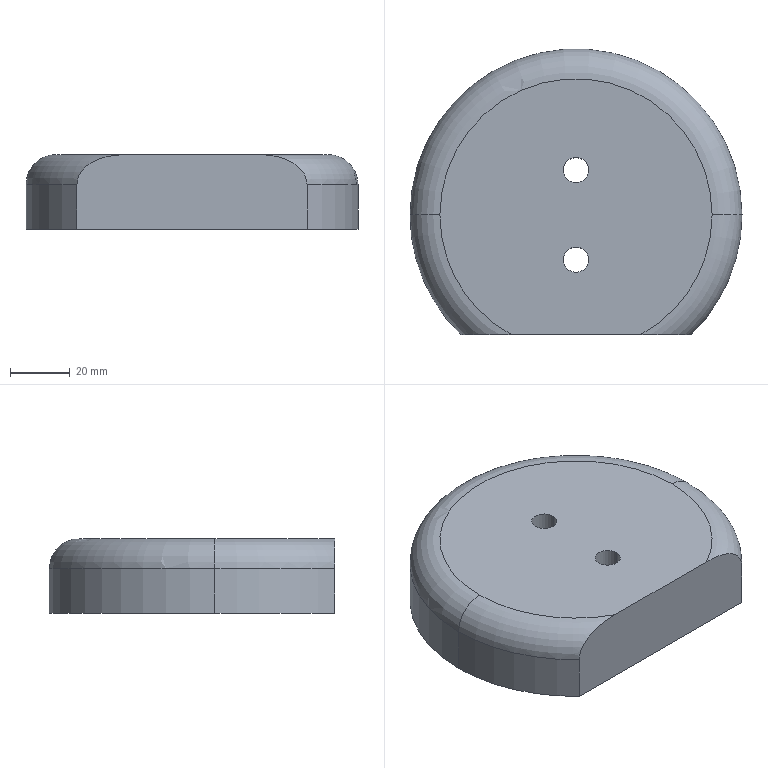Part | SolidWorks | features BaseBody 1 | 1 solid | 13 faces | box 111 x 95.5 x 25 mm | volume 213112 mm3 | cylinder 7 | plane 3 | torus 3 | commonest cylinder face diameters 8.4 x4 111 x3
STEP:
#1=CARTESIAN_POINT('',(-38.474,-40.,0.));
#2=VERTEX_POINT('',#1);
#3=CARTESIAN_POINT('',(38.474,-40.,0.));
#4=VERTEX_POINT('',#3);
#5=CARTESIAN_POINT('',(38.474,-40.,0.));
#6=DIRECTION('',(1.,0.,0.));
#7=VECTOR('',#6,1000.);
#8=LINE('',#5,#7);
#9=EDGE_CURVE('',#2,#4,#8,.T.);
#10=ORIENTED_EDGE('',*,*,#9,.T.);
#11=CARTESIAN_POINT('',(38.474,-40.,15.));
#12=VERTEX_POINT('',#11);
#13=CARTESIAN_POINT('',(38.474,-40.,-0.001));
#14=DIRECTION('',(0.,0.,1.));
#15=VECTOR('',#14,1000.);
#16=LINE('',#13,#15);
#17=EDGE_CURVE('',#4,#12,#16,.T.);
#18=ORIENTED_EDGE('',*,*,#17,.T.);
#19=CARTESIAN_POINT('',(21.685,-40.,25.));
#20=VERTEX_POINT('',#19);
#21=CARTESIAN_POINT('',(21.685,-40.,25.));
#22=CARTESIAN_POINT('',(22.606,-40.,25.));
#23=CARTESIAN_POINT('',(23.513,-40.,24.971));
#24=CARTESIAN_POINT('',(24.849,-40.,24.876));
#25=CARTESIAN_POINT('',(25.29,-40.,24.835));
#26=CARTESIAN_POINT('',(25.945,-40.,24.761));
#27=CARTESIAN_POINT('',(26.271,-40.,24.72));
#28=CARTESIAN_POINT('',(26.647,-40.,24.666));
#29=CARTESIAN_POINT('',(26.835,-40.,24.638));
#30=CARTESIAN_POINT('',(26.929,-40.,24.623));
#31=CARTESIAN_POINT('',(26.969,-40.,24.617));
#32=CARTESIAN_POINT('',(26.995,-40.,24.612));
#33=CARTESIAN_POINT('',(27.007,-40.,24.61));
#34=CARTESIAN_POINT('',(27.961,-40.,24.456));
#35=CARTESIAN_POINT('',(28.867,-40.,24.258));
#36=CARTESIAN_POINT('',(30.166,-40.,23.885));
#37=CARTESIAN_POINT('',(30.589,-40.,23.748));
#38=CARTESIAN_POINT('',(31.206,-40.,23.523));
#39=CARTESIAN_POINT('',(31.511,-40.,23.406));
#40=CARTESIAN_POINT('',(31.858,-40.,23.261));
#41=CARTESIAN_POINT('',(32.03,-40.,23.186));
#42=CARTESIAN_POINT('',(32.115,-40.,23.148));
#43=CARTESIAN_POINT('',(32.151,-40.,23.132));
#44=CARTESIAN_POINT('',(32.176,-40.,23.121));
#45=CARTESIAN_POINT('',(32.186,-40.,23.117));
#46=CARTESIAN_POINT('',(33.089,-40.,22.708));
#47=CARTESIAN_POINT('',(33.906,-40.,22.241));
#48=CARTESIAN_POINT('',(35.002,-40.,21.449));
#49=CARTESIAN_POINT('',(35.345,-40.,21.17));
#50=CARTESIAN_POINT('',(35.825,-40.,20.731));
#51=CARTESIAN_POINT('',(35.978,-40.,20.581));
#52=CARTESIAN_POINT('',(36.2,-40.,20.351));
#53=CARTESIAN_POINT('',(36.309,-40.,20.234));
#54=CARTESIAN_POINT('',(36.431,-40.,20.097));
#55=CARTESIAN_POINT('',(36.491,-40.,20.027));
#56=CARTESIAN_POINT('',(36.517,-40.,19.997));
#57=CARTESIAN_POINT('',(36.534,-40.,19.977));
#58=CARTESIAN_POINT('',(36.542,-40.,19.969));
#59=CARTESIAN_POINT('',(36.855,-40.,19.598));
#60=CARTESIAN_POINT('',(37.126,-40.,19.224));
#61=CARTESIAN_POINT('',(37.478,-40.,18.645));
#62=CARTESIAN_POINT('',(37.587,-40.,18.449));
#63=CARTESIAN_POINT('',(37.736,-40.,18.151));
#64=CARTESIAN_POINT('',(37.808,-40.,18.001));
#65=CARTESIAN_POINT('',(37.885,-40.,17.824));
#66=CARTESIAN_POINT('',(37.917,-40.,17.748));
#67=CARTESIAN_POINT('',(37.938,-40.,17.697));
#68=CARTESIAN_POINT('',(37.947,-40.,17.673));
#69=CARTESIAN_POINT('',(38.3,-40.,16.789));
#70=CARTESIAN_POINT('',(38.474,-40.,15.896));
#71=CARTESIAN_POINT('',(38.474,-40.,15.));
#72=B_SPLINE_CURVE_WITH_KNOTS('',3,(#21,#22,#23,#24,#25,#26,#27,#28,#29,#30,#31,#32,#33,#34,#35,#36,#37,#38,#39,#40,#41,#42,#43,#44,#45,#46,#47,#48,#49,#50,#51,#52,#53,#54,#55,#56,#57,#58,#59,#60,#61,#62,#63,#64,#65,#66,#67,#68,#69,#70,#71),.UNSPECIFIED.,.F.,.F.,(4,2,2,1,1,1,1,2,2,2,2,1,1,1,1,2,2,2,2,2,1,1,1,2,2,2,2,1,1,2,2,4),(0.,0.125,0.1875,0.2188,0.2344,0.2422,0.2461,0.248,0.25,0.375,0.4375,0.4688,0.4844,0.4922,0.4961,0.498,0.5,0.625,0.6875,0.7188,0.7344,0.7422,0.7461,0.748,0.75,0.8125,0.8437,0.8594,0.8672,0.8711,0.875,1.),.UNSPECIFIED.);
#73=EDGE_CURVE('',#20,#12,#72,.T.);
#74=ORIENTED_EDGE('',*,*,#73,.F.);
#75=CARTESIAN_POINT('',(-21.685,-40.,25.));
#76=VERTEX_POINT('',#75);
#77=CARTESIAN_POINT('',(38.474,-40.,25.));
#78=DIRECTION('',(-1.,0.,0.));
#79=VECTOR('',#78,1000.);
#80=LINE('',#77,#79);
#81=EDGE_CURVE('',#20,#76,#80,.T.);
#82=ORIENTED_EDGE('',*,*,#81,.T.);
#83=CARTESIAN_POINT('',(-38.474,-40.,15.));
#84=VERTEX_POINT('',#83);
#85=CARTESIAN_POINT('',(-38.474,-40.,15.));
#86=CARTESIAN_POINT('',(-38.474,-40.,15.879));
#87=CARTESIAN_POINT('',(-38.308,-39.999,16.75));
#88=CARTESIAN_POINT('',(-37.82,-39.999,18.005));
#89=CARTESIAN_POINT('',(-37.618,-39.999,18.414));
#90=CARTESIAN_POINT('',(-37.258,-40.,19.01));
#91=CARTESIAN_POINT('',(-37.128,-40.,19.205));
#92=CARTESIAN_POINT('',(-36.92,-40.,19.494));
#93=CARTESIAN_POINT('',(-36.813,-40.,19.636));
#94=CARTESIAN_POINT('',(-36.681,-40.,19.801));
#95=CARTESIAN_POINT('',(-36.614,-40.,19.882));
#96=CARTESIAN_POINT('',(-36.585,-40.,19.917));
#97=CARTESIAN_POINT('',(-36.566,-40.,19.94));
#98=CARTESIAN_POINT('',(-36.554,-40.,19.953));
#99=CARTESIAN_POINT('',(-36.004,-40.,20.603));
#100=CARTESIAN_POINT('',(-35.36,-40.,21.191));
#101=CARTESIAN_POINT('',(-34.263,-40.,21.982));
#102=CARTESIAN_POINT('',(-33.876,-40.,22.231));
#103=CARTESIAN_POINT('',(-33.265,-40.,22.58));
#104=CARTESIAN_POINT('',(-33.057,-40.,22.693));
#105=CARTESIAN_POINT('',(-32.737,-40.,22.856));
#106=CARTESIAN_POINT('',(-32.575,-40.,22.936));
#107=CARTESIAN_POINT('',(-32.383,-40.,23.026));
#108=CARTESIAN_POINT('',(-32.287,-40.,23.071));
#109=CARTESIAN_POINT('',(-32.245,-40.,23.09));
#110=CARTESIAN_POINT('',(-32.217,-40.,23.102));
#111=CARTESIAN_POINT('',(-32.202,-40.,23.109));
#112=CARTESIAN_POINT('',(-31.415,-40.,23.465));
#113=CARTESIAN_POINT('',(-30.591,-40.,23.763));
#114=CARTESIAN_POINT('',(-29.294,-40.,24.135));
#115=CARTESIAN_POINT('',(-28.852,-40.,24.247));
#116=CARTESIAN_POINT('',(-28.175,-40.,24.396));
#117=CARTESIAN_POINT('',(-27.833,-40.,24.466));
#118=CARTESIAN_POINT('',(-27.428,-40.,24.54));
#119=CARTESIAN_POINT('',(-27.224,-40.,24.575));
#120=CARTESIAN_POINT('',(-27.122,-40.,24.592));
#121=CARTESIAN_POINT('',(-27.078,-40.,24.599));
#122=CARTESIAN_POINT('',(-27.049,-40.,24.604));
#123=CARTESIAN_POINT('',(-27.033,-40.,24.606));
#124=CARTESIAN_POINT('',(-25.314,-40.,24.884));
#125=CARTESIAN_POINT('',(-23.527,-40.,25.));
#126=CARTESIAN_POINT('',(-21.685,-40.,25.));
#127=B_SPLINE_CURVE_WITH_KNOTS('',3,(#85,#86,#87,#88,#89,#90,#91,#92,#93,#94,#95,#96,#97,#98,#99,#100,#101,#102,#103,#104,#105,#106,#107,#108,#109,#110,#111,#112,#113,#114,#115,#116,#117,#118,#119,#120,#121,#122,#123,#124,#125,#126),.UNSPECIFIED.,.F.,.F.,(4,2,2,2,1,1,1,2,2,2,2,2,1,1,1,2,2,2,2,1,1,1,1,2,2,4),(0.,0.125,0.1875,0.2187,0.2344,0.2422,0.2461,0.248,0.25,0.375,0.4375,0.4687,0.4844,0.4922,0.4961,0.498,0.5,0.625,0.6875,0.7187,0.7344,0.7422,0.7461,0.748,0.75,1.),.UNSPECIFIED.);
#128=EDGE_CURVE('',#84,#76,#127,.T.);
#129=ORIENTED_EDGE('',*,*,#128,.F.);
#130=CARTESIAN_POINT('',(-38.474,-40.,-0.001));
#131=DIRECTION('',(0.,0.,1.));
#132=VECTOR('',#131,1000.);
#133=LINE('',#130,#132);
#134=EDGE_CURVE('',#2,#84,#133,.T.);
#135=ORIENTED_EDGE('',*,*,#134,.F.);
#136=EDGE_LOOP('',(#10,#18,#74,#82,#129,#135));
#137=FACE_OUTER_BOUND('',#136,.T.);
#138=CARTESIAN_POINT('',(38.474,-40.,-0.001));
#139=DIRECTION('',(0.,1.,0.));
#140=DIRECTION('',(1.,0.,0.));
#141=AXIS2_PLACEMENT_3D('',#138,#139,#140);
#142=PLANE('',#141);
#143=ADVANCED_FACE('',(#137),#142,.F.);
#144=CARTESIAN_POINT('',(-55.5,0.,15.));
#145=VERTEX_POINT('',#144);
#146=CARTESIAN_POINT('',(-45.5,0.,25.));
#147=VERTEX_POINT('',#146);
#148=CARTESIAN_POINT('',(-45.5,0.,15.));
#149=DIRECTION('',(0.,1.,0.));
#150=DIRECTION('',(-1.,0.,0.));
#151=AXIS2_PLACEMENT_3D('',#148,#149,#150);
#152=CIRCLE('',#151,10.);
#153=EDGE_CURVE('',#145,#147,#152,.T.);
#154=ORIENTED_EDGE('',*,*,#153,.F.);
#155=CARTESIAN_POINT('',(0.,0.,15.));
#156=DIRECTION('',(0.,0.,-1.));
#157=DIRECTION('',(1.,0.,0.));
#158=AXIS2_PLACEMENT_3D('',#155,#156,#157);
#159=CIRCLE('',#158,55.5);
#160=EDGE_CURVE('',#84,#145,#159,.T.);
#161=ORIENTED_EDGE('',*,*,#160,.F.);
#162=ORIENTED_EDGE('',*,*,#128,.T.);
#163=CARTESIAN_POINT('',(0.,0.,25.));
#164=DIRECTION('',(0.,0.,1.));
#165=DIRECTION('',(1.,0.,0.));
#166=AXIS2_PLACEMENT_3D('',#163,#164,#165);
#167=CIRCLE('',#166,45.5);
#168=EDGE_CURVE('',#147,#76,#167,.T.);
#169=ORIENTED_EDGE('',*,*,#168,.F.);
#170=EDGE_LOOP('',(#154,#161,#162,#169));
#171=FACE_OUTER_BOUND('',#170,.T.);
#172=CARTESIAN_POINT('',(0.,0.,15.));
#173=DIRECTION('',(0.,0.,1.));
#174=DIRECTION('',(1.,0.,0.));
#175=AXIS2_PLACEMENT_3D('',#172,#173,#174);
#176=TOROIDAL_SURFACE('',#175,45.5,10.);
#177=ADVANCED_FACE('',(#171),#176,.T.);
#178=CARTESIAN_POINT('',(-4.2,-15.,0.));
#179=VERTEX_POINT('',#178);
#180=CARTESIAN_POINT('',(-4.2,-15.,25.));
#181=VERTEX_POINT('',#180);
#182=CARTESIAN_POINT('',(-4.2,-15.,25.));
#183=DIRECTION('',(0.,0.,1.));
#184=VECTOR('',#183,1000.);
#185=LINE('',#182,#184);
#186=EDGE_CURVE('',#179,#181,#185,.T.);
#187=ORIENTED_EDGE('',*,*,#186,.F.);
#188=CARTESIAN_POINT('',(4.2,-15.,0.));
#189=VERTEX_POINT('',#188);
#190=CARTESIAN_POINT('',(0.,-15.,0.));
#191=DIRECTION('',(0.,0.,1.));
#192=DIRECTION('',(1.,0.,0.));
#193=AXIS2_PLACEMENT_3D('',#190,#191,#192);
#194=CIRCLE('',#193,4.2);
#195=EDGE_CURVE('',#189,#179,#194,.T.);
#196=ORIENTED_EDGE('',*,*,#195,.F.);
#197=CARTESIAN_POINT('',(4.2,-15.,25.));
#198=VERTEX_POINT('',#197);
#199=CARTESIAN_POINT('',(4.2,-15.,25.));
#200=DIRECTION('',(0.,0.,1.));
#201=VECTOR('',#200,1000.);
#202=LINE('',#199,#201);
#203=EDGE_CURVE('',#189,#198,#202,.T.);
#204=ORIENTED_EDGE('',*,*,#203,.T.);
#205=CARTESIAN_POINT('',(0.,-15.,25.));
#206=DIRECTION('',(0.,0.,1.));
#207=DIRECTION('',(1.,0.,0.));
#208=AXIS2_PLACEMENT_3D('',#205,#206,#207);
#209=CIRCLE('',#208,4.2);
#210=EDGE_CURVE('',#198,#181,#209,.T.);
#211=ORIENTED_EDGE('',*,*,#210,.T.);
#212=EDGE_LOOP('',(#187,#196,#204,#211));
#213=FACE_OUTER_BOUND('',#212,.T.);
#214=CARTESIAN_POINT('',(0.,-15.,25.));
#215=DIRECTION('',(0.,0.,1.));
#216=DIRECTION('',(1.,0.,0.));
#217=AXIS2_PLACEMENT_3D('',#214,#215,#216);
#218=CYLINDRICAL_SURFACE('',#217,4.2);
#219=ADVANCED_FACE('',(#213),#218,.F.);
#220=CARTESIAN_POINT('',(-4.2,15.,0.));
#221=VERTEX_POINT('',#220);
#222=CARTESIAN_POINT('',(-4.2,15.,25.));
#223=VERTEX_POINT('',#222);
#224=CARTESIAN_POINT('',(-4.2,15.,25.));
#225=DIRECTION('',(0.,0.,1.));
#226=VECTOR('',#225,1000.);
#227=LINE('',#224,#226);
#228=EDGE_CURVE('',#221,#223,#227,.T.);
#229=ORIENTED_EDGE('',*,*,#228,.F.);
#230=CARTESIAN_POINT('',(4.2,15.,0.));
#231=VERTEX_POINT('',#230);
#232=CARTESIAN_POINT('',(0.,15.,0.));
#233=DIRECTION('',(0.,0.,1.));
#234=DIRECTION('',(1.,0.,0.));
#235=AXIS2_PLACEMENT_3D('',#232,#233,#234);
#236=CIRCLE('',#235,4.2);
#237=EDGE_CURVE('',#231,#221,#236,.T.);
#238=ORIENTED_EDGE('',*,*,#237,.F.);
#239=CARTESIAN_POINT('',(4.2,15.,25.));
#240=VERTEX_POINT('',#239);
#241=CARTESIAN_POINT('',(4.2,15.,25.));
#242=DIRECTION('',(0.,0.,1.));
#243=VECTOR('',#242,1000.);
#244=LINE('',#241,#243);
#245=EDGE_CURVE('',#231,#240,#244,.T.);
#246=ORIENTED_EDGE('',*,*,#245,.T.);
#247=CARTESIAN_POINT('',(0.,15.,25.));
#248=DIRECTION('',(0.,0.,1.));
#249=DIRECTION('',(1.,0.,0.));
#250=AXIS2_PLACEMENT_3D('',#247,#248,#249);
#251=CIRCLE('',#250,4.2);
#252=EDGE_CURVE('',#240,#223,#251,.T.);
#253=ORIENTED_EDGE('',*,*,#252,.T.);
#254=EDGE_LOOP('',(#229,#238,#246,#253));
#255=FACE_OUTER_BOUND('',#254,.T.);
#256=CARTESIAN_POINT('',(0.,15.,25.));
#257=DIRECTION('',(0.,0.,1.));
#258=DIRECTION('',(1.,0.,0.));
#259=AXIS2_PLACEMENT_3D('',#256,#257,#258);
#260=CYLINDRICAL_SURFACE('',#259,4.2);
#261=ADVANCED_FACE('',(#255),#260,.F.);
#262=ORIENTED_EDGE('',*,*,#237,.T.);
#263=CARTESIAN_POINT('',(0.,15.,0.));
#264=DIRECTION('',(0.,0.,1.));
#265=DIRECTION('',(1.,0.,0.));
#266=AXIS2_PLACEMENT_3D('',#263,#264,#265);
#267=CIRCLE('',#266,4.2);
#268=EDGE_CURVE('',#221,#231,#267,.T.);
#269=ORIENTED_EDGE('',*,*,#268,.T.);
#270=EDGE_LOOP('',(#262,#269));
#271=FACE_BOUND('',#270,.T.);
#272=ORIENTED_EDGE('',*,*,#195,.T.);
#273=CARTESIAN_POINT('',(0.,-15.,0.));
#274=DIRECTION('',(0.,0.,1.));
#275=DIRECTION('',(1.,0.,0.));
#276=AXIS2_PLACEMENT_3D('',#273,#274,#275);
#277=CIRCLE('',#276,4.2);
#278=EDGE_CURVE('',#179,#189,#277,.T.);
#279=ORIENTED_EDGE('',*,*,#278,.T.);
#280=EDGE_LOOP('',(#272,#279));
#281=FACE_BOUND('',#280,.T.);
#282=CARTESIAN_POINT('',(55.5,0.,0.));
#283=VERTEX_POINT('',#282);
#284=CARTESIAN_POINT('',(0.,0.,0.));
#285=DIRECTION('',(0.,0.,1.));
#286=DIRECTION('',(1.,0.,0.));
#287=AXIS2_PLACEMENT_3D('',#284,#285,#286);
#288=CIRCLE('',#287,55.5);
#289=EDGE_CURVE('',#4,#283,#288,.T.);
#290=ORIENTED_EDGE('',*,*,#289,.F.);
#291=ORIENTED_EDGE('',*,*,#9,.F.);
#292=CARTESIAN_POINT('',(-55.5,0.,0.));
#293=VERTEX_POINT('',#292);
#294=CARTESIAN_POINT('',(0.,0.,0.));
#295=DIRECTION('',(0.,0.,1.));
#296=DIRECTION('',(1.,0.,0.));
#297=AXIS2_PLACEMENT_3D('',#294,#295,#296);
#298=CIRCLE('',#297,55.5);
#299=EDGE_CURVE('',#293,#2,#298,.T.);
#300=ORIENTED_EDGE('',*,*,#299,.F.);
#301=CARTESIAN_POINT('',(0.,0.,0.));
#302=DIRECTION('',(0.,0.,1.));
#303=DIRECTION('',(1.,0.,0.));
#304=AXIS2_PLACEMENT_3D('',#301,#302,#303);
#305=CIRCLE('',#304,55.5);
#306=EDGE_CURVE('',#283,#293,#305,.T.);
#307=ORIENTED_EDGE('',*,*,#306,.F.);
#308=EDGE_LOOP('',(#290,#291,#300,#307));
#309=FACE_OUTER_BOUND('',#308,.T.);
#310=CARTESIAN_POINT('',(0.,0.,0.));
#311=DIRECTION('',(0.,0.,1.));
#312=DIRECTION('',(1.,0.,0.));
#313=AXIS2_PLACEMENT_3D('',#310,#311,#312);
#314=PLANE('',#313);
#315=ADVANCED_FACE('',(#271,#281,#309),#314,.F.);
#316=ORIENTED_EDGE('',*,*,#252,.F.);
#317=CARTESIAN_POINT('',(0.,15.,25.));
#318=DIRECTION('',(0.,0.,1.));
#319=DIRECTION('',(1.,0.,0.));
#320=AXIS2_PLACEMENT_3D('',#317,#318,#319);
#321=CIRCLE('',#320,4.2);
#322=EDGE_CURVE('',#223,#240,#321,.T.);
#323=ORIENTED_EDGE('',*,*,#322,.F.);
#324=EDGE_LOOP('',(#316,#323));
#325=FACE_BOUND('',#324,.T.);
#326=ORIENTED_EDGE('',*,*,#210,.F.);
#327=CARTESIAN_POINT('',(0.,-15.,25.));
#328=DIRECTION('',(0.,0.,1.));
#329=DIRECTION('',(1.,0.,0.));
#330=AXIS2_PLACEMENT_3D('',#327,#328,#329);
#331=CIRCLE('',#330,4.2);
#332=EDGE_CURVE('',#181,#198,#331,.T.);
#333=ORIENTED_EDGE('',*,*,#332,.F.);
#334=EDGE_LOOP('',(#326,#333));
#335=FACE_BOUND('',#334,.T.);
#336=ORIENTED_EDGE('',*,*,#81,.F.);
#337=CARTESIAN_POINT('',(45.5,0.,25.));
#338=VERTEX_POINT('',#337);
#339=CARTESIAN_POINT('',(0.,0.,25.));
#340=DIRECTION('',(0.,0.,1.));
#341=DIRECTION('',(1.,0.,0.));
#342=AXIS2_PLACEMENT_3D('',#339,#340,#341);
#343=CIRCLE('',#342,45.5);
#344=EDGE_CURVE('',#20,#338,#343,.T.);
#345=ORIENTED_EDGE('',*,*,#344,.T.);
#346=CARTESIAN_POINT('',(0.,0.,25.));
#347=DIRECTION('',(0.,0.,1.));
#348=DIRECTION('',(1.,0.,0.));
#349=AXIS2_PLACEMENT_3D('',#346,#347,#348);
#350=CIRCLE('',#349,45.5);
#351=EDGE_CURVE('',#338,#147,#350,.T.);
#352=ORIENTED_EDGE('',*,*,#351,.T.);
#353=ORIENTED_EDGE('',*,*,#168,.T.);
#354=EDGE_LOOP('',(#336,#345,#352,#353));
#355=FACE_OUTER_BOUND('',#354,.T.);
#356=CARTESIAN_POINT('',(0.,0.,25.));
#357=DIRECTION('',(0.,0.,1.));
#358=DIRECTION('',(1.,0.,0.));
#359=AXIS2_PLACEMENT_3D('',#356,#357,#358);
#360=PLANE('',#359);
#361=ADVANCED_FACE('',(#325,#335,#355),#360,.T.);
#362=CARTESIAN_POINT('',(55.5,0.,15.));
#363=VERTEX_POINT('',#362);
#364=CARTESIAN_POINT('',(55.5,0.,25.));
#365=DIRECTION('',(0.,0.,-1.));
#366=VECTOR('',#365,1000.);
#367=LINE('',#364,#366);
#368=EDGE_CURVE('',#363,#283,#367,.T.);
#369=ORIENTED_EDGE('',*,*,#368,.F.);
#370=CARTESIAN_POINT('',(0.,0.,15.));
#371=DIRECTION('',(0.,0.,-1.));
#372=DIRECTION('',(1.,0.,0.));
#373=AXIS2_PLACEMENT_3D('',#370,#371,#372);
#374=CIRCLE('',#373,55.5);
#375=EDGE_CURVE('',#363,#12,#374,.T.);
#376=ORIENTED_EDGE('',*,*,#375,.T.);
#377=ORIENTED_EDGE('',*,*,#17,.F.);
#378=ORIENTED_EDGE('',*,*,#289,.T.);
#379=EDGE_LOOP('',(#369,#376,#377,#378));
#380=FACE_OUTER_BOUND('',#379,.T.);
#381=CARTESIAN_POINT('',(0.,0.,25.));
#382=DIRECTION('',(0.,0.,-1.));
#383=DIRECTION('',(-1.,0.,0.));
#384=AXIS2_PLACEMENT_3D('',#381,#382,#383);
#385=CYLINDRICAL_SURFACE('',#384,55.5);
#386=ADVANCED_FACE('',(#380),#385,.T.);
#387=ORIENTED_EDGE('',*,*,#160,.T.);
#388=CARTESIAN_POINT('',(-55.5,0.,25.));
#389=DIRECTION('',(0.,0.,-1.));
#390=VECTOR('',#389,1000.);
#391=LINE('',#388,#390);
#392=EDGE_CURVE('',#145,#293,#391,.T.);
#393=ORIENTED_EDGE('',*,*,#392,.T.);
#394=ORIENTED_EDGE('',*,*,#299,.T.);
#395=ORIENTED_EDGE('',*,*,#134,.T.);
#396=EDGE_LOOP('',(#387,#393,#394,#395));
#397=FACE_OUTER_BOUND('',#396,.T.);
#398=CARTESIAN_POINT('',(0.,0.,25.));
#399=DIRECTION('',(0.,0.,-1.));
#400=DIRECTION('',(-1.,0.,0.));
#401=AXIS2_PLACEMENT_3D('',#398,#399,#400);
#402=CYLINDRICAL_SURFACE('',#401,55.5);
#403=ADVANCED_FACE('',(#397),#402,.T.);
#404=CARTESIAN_POINT('',(0.,0.,15.));
#405=DIRECTION('',(0.,0.,-1.));
#406=DIRECTION('',(1.,0.,0.));
#407=AXIS2_PLACEMENT_3D('',#404,#405,#406);
#408=CIRCLE('',#407,55.5);
#409=EDGE_CURVE('',#145,#363,#408,.T.);
#410=ORIENTED_EDGE('',*,*,#409,.T.);
#411=ORIENTED_EDGE('',*,*,#368,.T.);
#412=ORIENTED_EDGE('',*,*,#306,.T.);
#413=ORIENTED_EDGE('',*,*,#392,.F.);
#414=EDGE_LOOP('',(#410,#411,#412,#413));
#415=FACE_OUTER_BOUND('',#414,.T.);
#416=CARTESIAN_POINT('',(0.,0.,25.));
#417=DIRECTION('',(0.,0.,-1.));
#418=DIRECTION('',(-1.,0.,0.));
#419=AXIS2_PLACEMENT_3D('',#416,#417,#418);
#420=CYLINDRICAL_SURFACE('',#419,55.5);
#421=ADVANCED_FACE('',(#415),#420,.T.);
#422=ORIENTED_EDGE('',*,*,#268,.F.);
#423=ORIENTED_EDGE('',*,*,#228,.T.);
#424=ORIENTED_EDGE('',*,*,#322,.T.);
#425=ORIENTED_EDGE('',*,*,#245,.F.);
#426=EDGE_LOOP('',(#422,#423,#424,#425));
#427=FACE_OUTER_BOUND('',#426,.T.);
#428=CARTESIAN_POINT('',(0.,15.,25.));
#429=DIRECTION('',(0.,0.,1.));
#430=DIRECTION('',(1.,0.,0.));
#431=AXIS2_PLACEMENT_3D('',#428,#429,#430);
#432=CYLINDRICAL_SURFACE('',#431,4.2);
#433=ADVANCED_FACE('',(#427),#432,.F.);
#434=ORIENTED_EDGE('',*,*,#278,.F.);
#435=ORIENTED_EDGE('',*,*,#186,.T.);
#436=ORIENTED_EDGE('',*,*,#332,.T.);
#437=ORIENTED_EDGE('',*,*,#203,.F.);
#438=EDGE_LOOP('',(#434,#435,#436,#437));
#439=FACE_OUTER_BOUND('',#438,.T.);
#440=CARTESIAN_POINT('',(0.,-15.,25.));
#441=DIRECTION('',(0.,0.,1.));
#442=DIRECTION('',(1.,0.,0.));
#443=AXIS2_PLACEMENT_3D('',#440,#441,#442);
#444=CYLINDRICAL_SURFACE('',#443,4.2);
#445=ADVANCED_FACE('',(#439),#444,.F.);
#446=ORIENTED_EDGE('',*,*,#375,.F.);
#447=CARTESIAN_POINT('',(45.5,0.,15.));
#448=DIRECTION('',(0.,-1.,0.));
#449=DIRECTION('',(0.,0.,-1.));
#450=AXIS2_PLACEMENT_3D('',#447,#448,#449);
#451=CIRCLE('',#450,10.);
#452=EDGE_CURVE('',#363,#338,#451,.T.);
#453=ORIENTED_EDGE('',*,*,#452,.T.);
#454=ORIENTED_EDGE('',*,*,#344,.F.);
#455=ORIENTED_EDGE('',*,*,#73,.T.);
#456=EDGE_LOOP('',(#446,#453,#454,#455));
#457=FACE_OUTER_BOUND('',#456,.T.);
#458=CARTESIAN_POINT('',(0.,0.,15.));
#459=DIRECTION('',(0.,0.,1.));
#460=DIRECTION('',(1.,0.,0.));
#461=AXIS2_PLACEMENT_3D('',#458,#459,#460);
#462=TOROIDAL_SURFACE('',#461,45.5,10.);
#463=ADVANCED_FACE('',(#457),#462,.T.);
#464=ORIENTED_EDGE('',*,*,#409,.F.);
#465=ORIENTED_EDGE('',*,*,#153,.T.);
#466=ORIENTED_EDGE('',*,*,#351,.F.);
#467=ORIENTED_EDGE('',*,*,#452,.F.);
#468=EDGE_LOOP('',(#464,#465,#466,#467));
#469=FACE_OUTER_BOUND('',#468,.T.);
#470=CARTESIAN_POINT('',(0.,0.,15.));
#471=DIRECTION('',(0.,0.,1.));
#472=DIRECTION('',(1.,0.,0.));
#473=AXIS2_PLACEMENT_3D('',#470,#471,#472);
#474=TOROIDAL_SURFACE('',#473,45.5,10.);
#475=ADVANCED_FACE('',(#469),#474,.T.);
#476=CLOSED_SHELL('',(#143,#177,#219,#261,#315,#361,#386,#403,#421,#433,#445,#463,#475));
#477=MANIFOLD_SOLID_BREP('',#476);
#478=CARTESIAN_POINT('',(0.,0.,0.));
#479=DIRECTION('',(0.,0.,1.));
#480=DIRECTION('',(1.,0.,0.));
#481=AXIS2_PLACEMENT_3D('',#478,#479,#480);
#482=(LENGTH_UNIT()NAMED_UNIT(*)SI_UNIT(.MILLI.,.METRE.));
#483=UNCERTAINTY_MEASURE_WITH_UNIT(LENGTH_MEASURE(0.00001),#482,'','');
#484=(NAMED_UNIT(*)PLANE_ANGLE_UNIT()SI_UNIT($,.RADIAN.));
#485=(NAMED_UNIT(*)SI_UNIT($,.STERADIAN.)SOLID_ANGLE_UNIT());
#486=(GEOMETRIC_REPRESENTATION_CONTEXT(3)GLOBAL_UNCERTAINTY_ASSIGNED_CONTEXT((#483))GLOBAL_UNIT_ASSIGNED_CONTEXT((#482,#484,#485))REPRESENTATION_CONTEXT('',''));
#487=ADVANCED_BREP_SHAPE_REPRESENTATION('',(#477,#481),#486);